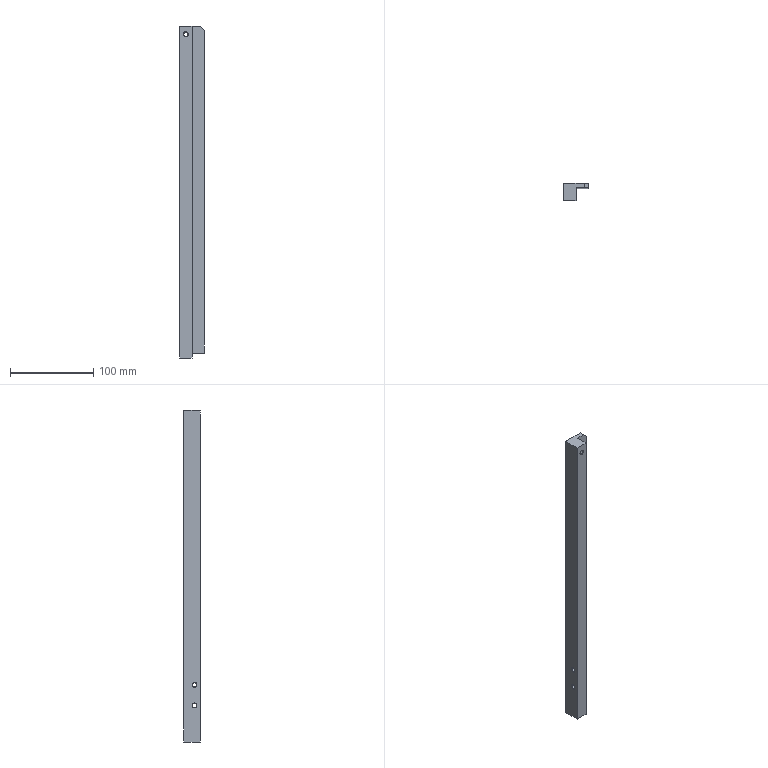Part | STEP file | Tube necking machine_id198_x_t | 1 solid | 19 faces | box 30 x 20 x 400 mm | volume 151442 mm3 | plane 10 | cone 6 | cylinder 3 | commonest cylinder face diameters 5 x3